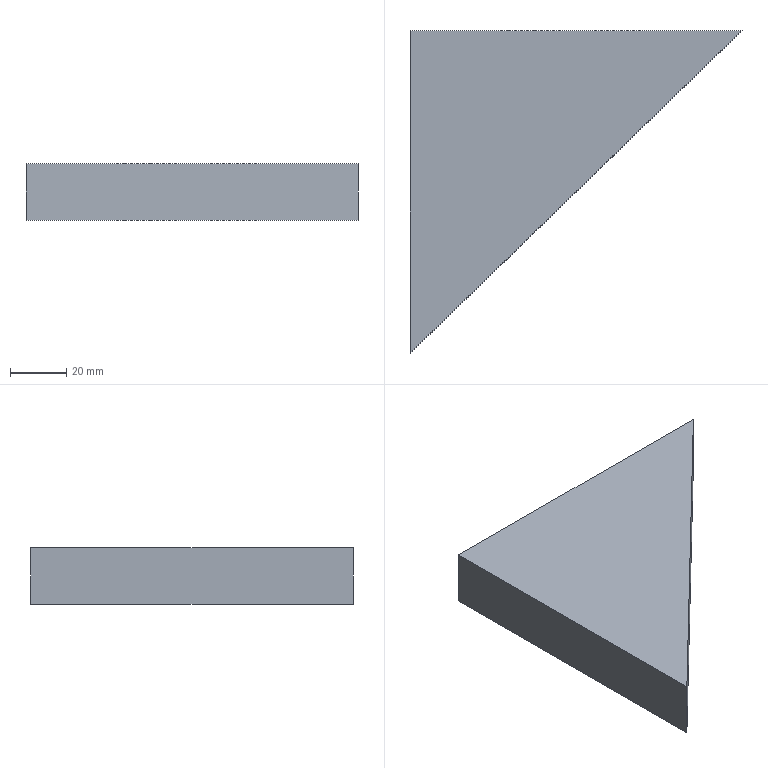Part | STEP file | 1 solid | 5 faces | box 117.801 x 114.536 x 20 mm | volume 134925 mm3 | plane 5
STEP:
#1=CARTESIAN_POINT('',(0.,0.,0.));
#2=DIRECTION('',(0.,0.,1.));
#3=DIRECTION('',(1.,0.,0.));
#4=AXIS2_PLACEMENT_3D('',#1,#2,#3);
#5=CARTESIAN_POINT('',(-480.,430.,-10.));
#6=VERTEX_POINT('',#5);
#7=CARTESIAN_POINT('',(-480.,315.464,-10.));
#8=VERTEX_POINT('',#7);
#9=CARTESIAN_POINT('',(-480.,430.,-10.));
#10=DIRECTION('',(0.,-1.,0.));
#11=VECTOR('',#10,1.);
#12=LINE('',#9,#11);
#13=CARTESIAN_POINT('',(-480.,430.,10.));
#14=DIRECTION('',(1.,0.,0.));
#15=DIRECTION('',(0.,0.,-1.));
#16=AXIS2_PLACEMENT_3D('',#13,#14,#15);
#17=PLANE('',#16);
#18=CARTESIAN_POINT('',(20.,0.));
#19=DIRECTION('',(0.,-1.));
#20=VECTOR('',#19,1.);
#21=LINE('',#18,#20);
#22=(GEOMETRIC_REPRESENTATION_CONTEXT(2)PARAMETRIC_REPRESENTATION_CONTEXT()REPRESENTATION_CONTEXT('',''));
#23=DEFINITIONAL_REPRESENTATION('',(#21),#22);
#24=PCURVE('',#17,#23);
#25=CARTESIAN_POINT('',(0.,0.,-10.));
#26=DIRECTION('',(0.,0.,-1.));
#27=DIRECTION('',(-1.,0.,0.));
#28=AXIS2_PLACEMENT_3D('',#25,#26,#27);
#29=PLANE('',#28);
#30=CARTESIAN_POINT('',(480.,430.));
#31=DIRECTION('',(0.,-1.));
#32=VECTOR('',#31,1.);
#33=LINE('',#30,#32);
#34=(GEOMETRIC_REPRESENTATION_CONTEXT(2)PARAMETRIC_REPRESENTATION_CONTEXT()REPRESENTATION_CONTEXT('',''));
#35=DEFINITIONAL_REPRESENTATION('',(#33),#34);
#36=PCURVE('',#29,#35);
#37=SURFACE_CURVE('',#12,(#24,#36),.PCURVE_S1.);
#38=EDGE_CURVE('',#6,#8,#37,.T.);
#39=ORIENTED_EDGE('',*,*,#38,.T.);
#40=CARTESIAN_POINT('',(-480.,315.464,10.));
#41=VERTEX_POINT('',#40);
#42=CARTESIAN_POINT('',(-480.,315.464,10.));
#43=DIRECTION('',(0.,0.,-1.));
#44=VECTOR('',#43,1.);
#45=LINE('',#42,#44);
#46=CARTESIAN_POINT('',(0.,-114.536));
#47=DIRECTION('',(1.,0.));
#48=VECTOR('',#47,1.);
#49=LINE('',#46,#48);
#50=(GEOMETRIC_REPRESENTATION_CONTEXT(2)PARAMETRIC_REPRESENTATION_CONTEXT()REPRESENTATION_CONTEXT('',''));
#51=DEFINITIONAL_REPRESENTATION('',(#49),#50);
#52=PCURVE('',#17,#51);
#53=CARTESIAN_POINT('',(-480.,315.464,10.));
#54=DIRECTION('',(-0.6971,0.717,0.));
#55=DIRECTION('',(-0.717,-0.6971,0.));
#56=AXIS2_PLACEMENT_3D('',#53,#54,#55);
#57=PLANE('',#56);
#58=CARTESIAN_POINT('',(0.,0.));
#59=DIRECTION('',(0.,-1.));
#60=VECTOR('',#59,1.);
#61=LINE('',#58,#60);
#62=(GEOMETRIC_REPRESENTATION_CONTEXT(2)PARAMETRIC_REPRESENTATION_CONTEXT()REPRESENTATION_CONTEXT('',''));
#63=DEFINITIONAL_REPRESENTATION('',(#61),#62);
#64=PCURVE('',#57,#63);
#65=SURFACE_CURVE('',#45,(#52,#64),.PCURVE_S1.);
#66=EDGE_CURVE('',#41,#8,#65,.T.);
#67=ORIENTED_EDGE('',*,*,#66,.F.);
#68=CARTESIAN_POINT('',(-480.,430.,10.));
#69=VERTEX_POINT('',#68);
#70=CARTESIAN_POINT('',(-480.,430.,10.));
#71=DIRECTION('',(0.,-1.,0.));
#72=VECTOR('',#71,1.);
#73=LINE('',#70,#72);
#74=CARTESIAN_POINT('',(0.,0.));
#75=DIRECTION('',(0.,-1.));
#76=VECTOR('',#75,1.);
#77=LINE('',#74,#76);
#78=(GEOMETRIC_REPRESENTATION_CONTEXT(2)PARAMETRIC_REPRESENTATION_CONTEXT()REPRESENTATION_CONTEXT('',''));
#79=DEFINITIONAL_REPRESENTATION('',(#77),#78);
#80=PCURVE('',#17,#79);
#81=CARTESIAN_POINT('',(0.,0.,10.));
#82=DIRECTION('',(0.,0.,-1.));
#83=DIRECTION('',(-1.,0.,0.));
#84=AXIS2_PLACEMENT_3D('',#81,#82,#83);
#85=PLANE('',#84);
#86=CARTESIAN_POINT('',(480.,430.));
#87=DIRECTION('',(0.,-1.));
#88=VECTOR('',#87,1.);
#89=LINE('',#86,#88);
#90=(GEOMETRIC_REPRESENTATION_CONTEXT(2)PARAMETRIC_REPRESENTATION_CONTEXT()REPRESENTATION_CONTEXT('',''));
#91=DEFINITIONAL_REPRESENTATION('',(#89),#90);
#92=PCURVE('',#85,#91);
#93=SURFACE_CURVE('',#73,(#80,#92),.PCURVE_S1.);
#94=EDGE_CURVE('',#69,#41,#93,.T.);
#95=ORIENTED_EDGE('',*,*,#94,.F.);
#96=CARTESIAN_POINT('',(-480.,430.,10.));
#97=DIRECTION('',(0.,0.,-1.));
#98=VECTOR('',#97,1.);
#99=LINE('',#96,#98);
#100=CARTESIAN_POINT('',(0.,0.));
#101=DIRECTION('',(1.,0.));
#102=VECTOR('',#101,1.);
#103=LINE('',#100,#102);
#104=(GEOMETRIC_REPRESENTATION_CONTEXT(2)PARAMETRIC_REPRESENTATION_CONTEXT()REPRESENTATION_CONTEXT('',''));
#105=DEFINITIONAL_REPRESENTATION('',(#103),#104);
#106=PCURVE('',#17,#105);
#107=CARTESIAN_POINT('',(-362.199,430.,10.));
#108=DIRECTION('',(0.,-1.,0.));
#109=DIRECTION('',(0.,0.,-1.));
#110=AXIS2_PLACEMENT_3D('',#107,#108,#109);
#111=PLANE('',#110);
#112=CARTESIAN_POINT('',(0.,-117.801));
#113=DIRECTION('',(1.,0.));
#114=VECTOR('',#113,1.);
#115=LINE('',#112,#114);
#116=(GEOMETRIC_REPRESENTATION_CONTEXT(2)PARAMETRIC_REPRESENTATION_CONTEXT()REPRESENTATION_CONTEXT('',''));
#117=DEFINITIONAL_REPRESENTATION('',(#115),#116);
#118=PCURVE('',#111,#117);
#119=SURFACE_CURVE('',#99,(#106,#118),.PCURVE_S1.);
#120=EDGE_CURVE('',#69,#6,#119,.T.);
#121=ORIENTED_EDGE('',*,*,#120,.T.);
#122=EDGE_LOOP('',(#39,#67,#95,#121));
#123=FACE_BOUND('',#122,.T.);
#124=ADVANCED_FACE('',(#123),#17,.F.);
#125=CARTESIAN_POINT('',(-362.199,430.,-10.));
#126=VERTEX_POINT('',#125);
#127=CARTESIAN_POINT('',(-480.,315.464,-10.));
#128=DIRECTION('',(0.717,0.6971,0.));
#129=VECTOR('',#128,1.);
#130=LINE('',#127,#129);
#131=CARTESIAN_POINT('',(0.,-20.));
#132=DIRECTION('',(-1.,0.));
#133=VECTOR('',#132,1.);
#134=LINE('',#131,#133);
#135=(GEOMETRIC_REPRESENTATION_CONTEXT(2)PARAMETRIC_REPRESENTATION_CONTEXT()REPRESENTATION_CONTEXT('',''));
#136=DEFINITIONAL_REPRESENTATION('',(#134),#135);
#137=PCURVE('',#57,#136);
#138=CARTESIAN_POINT('',(480.,315.464));
#139=DIRECTION('',(-0.717,0.6971));
#140=VECTOR('',#139,1.);
#141=LINE('',#138,#140);
#142=(GEOMETRIC_REPRESENTATION_CONTEXT(2)PARAMETRIC_REPRESENTATION_CONTEXT()REPRESENTATION_CONTEXT('',''));
#143=DEFINITIONAL_REPRESENTATION('',(#141),#142);
#144=PCURVE('',#29,#143);
#145=SURFACE_CURVE('',#130,(#137,#144),.PCURVE_S1.);
#146=EDGE_CURVE('',#8,#126,#145,.T.);
#147=ORIENTED_EDGE('',*,*,#146,.T.);
#148=CARTESIAN_POINT('',(-362.199,430.,10.));
#149=VERTEX_POINT('',#148);
#150=CARTESIAN_POINT('',(-362.199,430.,10.));
#151=DIRECTION('',(0.,0.,-1.));
#152=VECTOR('',#151,1.);
#153=LINE('',#150,#152);
#154=CARTESIAN_POINT('',(-164.304,0.));
#155=DIRECTION('',(0.,-1.));
#156=VECTOR('',#155,1.);
#157=LINE('',#154,#156);
#158=(GEOMETRIC_REPRESENTATION_CONTEXT(2)PARAMETRIC_REPRESENTATION_CONTEXT()REPRESENTATION_CONTEXT('',''));
#159=DEFINITIONAL_REPRESENTATION('',(#157),#158);
#160=PCURVE('',#57,#159);
#161=CARTESIAN_POINT('',(0.,0.));
#162=DIRECTION('',(1.,0.));
#163=VECTOR('',#162,1.);
#164=LINE('',#161,#163);
#165=(GEOMETRIC_REPRESENTATION_CONTEXT(2)PARAMETRIC_REPRESENTATION_CONTEXT()REPRESENTATION_CONTEXT('',''));
#166=DEFINITIONAL_REPRESENTATION('',(#164),#165);
#167=PCURVE('',#111,#166);
#168=SURFACE_CURVE('',#153,(#160,#167),.PCURVE_S1.);
#169=EDGE_CURVE('',#149,#126,#168,.T.);
#170=ORIENTED_EDGE('',*,*,#169,.F.);
#171=CARTESIAN_POINT('',(-480.,315.464,10.));
#172=DIRECTION('',(0.717,0.6971,0.));
#173=VECTOR('',#172,1.);
#174=LINE('',#171,#173);
#175=CARTESIAN_POINT('',(0.,0.));
#176=DIRECTION('',(-1.,0.));
#177=VECTOR('',#176,1.);
#178=LINE('',#175,#177);
#179=(GEOMETRIC_REPRESENTATION_CONTEXT(2)PARAMETRIC_REPRESENTATION_CONTEXT()REPRESENTATION_CONTEXT('',''));
#180=DEFINITIONAL_REPRESENTATION('',(#178),#179);
#181=PCURVE('',#57,#180);
#182=CARTESIAN_POINT('',(480.,315.464));
#183=DIRECTION('',(-0.717,0.6971));
#184=VECTOR('',#183,1.);
#185=LINE('',#182,#184);
#186=(GEOMETRIC_REPRESENTATION_CONTEXT(2)PARAMETRIC_REPRESENTATION_CONTEXT()REPRESENTATION_CONTEXT('',''));
#187=DEFINITIONAL_REPRESENTATION('',(#185),#186);
#188=PCURVE('',#85,#187);
#189=SURFACE_CURVE('',#174,(#181,#188),.PCURVE_S1.);
#190=EDGE_CURVE('',#41,#149,#189,.T.);
#191=ORIENTED_EDGE('',*,*,#190,.F.);
#192=ORIENTED_EDGE('',*,*,#66,.T.);
#193=EDGE_LOOP('',(#147,#170,#191,#192));
#194=FACE_BOUND('',#193,.T.);
#195=ADVANCED_FACE('',(#194),#57,.F.);
#196=CARTESIAN_POINT('',(-362.199,430.,-10.));
#197=DIRECTION('',(-1.,0.,0.));
#198=VECTOR('',#197,1.);
#199=LINE('',#196,#198);
#200=CARTESIAN_POINT('',(20.,0.));
#201=DIRECTION('',(0.,-1.));
#202=VECTOR('',#201,1.);
#203=LINE('',#200,#202);
#204=(GEOMETRIC_REPRESENTATION_CONTEXT(2)PARAMETRIC_REPRESENTATION_CONTEXT()REPRESENTATION_CONTEXT('',''));
#205=DEFINITIONAL_REPRESENTATION('',(#203),#204);
#206=PCURVE('',#111,#205);
#207=CARTESIAN_POINT('',(362.199,430.));
#208=DIRECTION('',(1.,0.));
#209=VECTOR('',#208,1.);
#210=LINE('',#207,#209);
#211=(GEOMETRIC_REPRESENTATION_CONTEXT(2)PARAMETRIC_REPRESENTATION_CONTEXT()REPRESENTATION_CONTEXT('',''));
#212=DEFINITIONAL_REPRESENTATION('',(#210),#211);
#213=PCURVE('',#29,#212);
#214=SURFACE_CURVE('',#199,(#206,#213),.PCURVE_S1.);
#215=EDGE_CURVE('',#126,#6,#214,.T.);
#216=ORIENTED_EDGE('',*,*,#215,.T.);
#217=ORIENTED_EDGE('',*,*,#120,.F.);
#218=CARTESIAN_POINT('',(-362.199,430.,10.));
#219=DIRECTION('',(-1.,0.,0.));
#220=VECTOR('',#219,1.);
#221=LINE('',#218,#220);
#222=CARTESIAN_POINT('',(0.,0.));
#223=DIRECTION('',(0.,-1.));
#224=VECTOR('',#223,1.);
#225=LINE('',#222,#224);
#226=(GEOMETRIC_REPRESENTATION_CONTEXT(2)PARAMETRIC_REPRESENTATION_CONTEXT()REPRESENTATION_CONTEXT('',''));
#227=DEFINITIONAL_REPRESENTATION('',(#225),#226);
#228=PCURVE('',#111,#227);
#229=CARTESIAN_POINT('',(362.199,430.));
#230=DIRECTION('',(1.,0.));
#231=VECTOR('',#230,1.);
#232=LINE('',#229,#231);
#233=(GEOMETRIC_REPRESENTATION_CONTEXT(2)PARAMETRIC_REPRESENTATION_CONTEXT()REPRESENTATION_CONTEXT('',''));
#234=DEFINITIONAL_REPRESENTATION('',(#232),#233);
#235=PCURVE('',#85,#234);
#236=SURFACE_CURVE('',#221,(#228,#235),.PCURVE_S1.);
#237=EDGE_CURVE('',#149,#69,#236,.T.);
#238=ORIENTED_EDGE('',*,*,#237,.F.);
#239=ORIENTED_EDGE('',*,*,#169,.T.);
#240=EDGE_LOOP('',(#216,#217,#238,#239));
#241=FACE_BOUND('',#240,.T.);
#242=ADVANCED_FACE('',(#241),#111,.F.);
#243=ORIENTED_EDGE('',*,*,#94,.T.);
#244=ORIENTED_EDGE('',*,*,#190,.T.);
#245=ORIENTED_EDGE('',*,*,#237,.T.);
#246=EDGE_LOOP('',(#243,#244,#245));
#247=FACE_BOUND('',#246,.T.);
#248=ADVANCED_FACE('',(#247),#85,.F.);
#249=ORIENTED_EDGE('',*,*,#38,.F.);
#250=ORIENTED_EDGE('',*,*,#215,.F.);
#251=ORIENTED_EDGE('',*,*,#146,.F.);
#252=EDGE_LOOP('',(#249,#250,#251));
#253=FACE_BOUND('',#252,.T.);
#254=ADVANCED_FACE('',(#253),#29,.T.);
#255=CLOSED_SHELL('',(#124,#195,#242,#248,#254));
#256=MANIFOLD_SOLID_BREP('',#255);
#257=(LENGTH_UNIT()NAMED_UNIT(*)SI_UNIT(.MILLI.,.METRE.));
#258=UNCERTAINTY_MEASURE_WITH_UNIT(LENGTH_MEASURE(0.0000001),#257,'','');
#259=(NAMED_UNIT(*)PLANE_ANGLE_UNIT()SI_UNIT($,.RADIAN.));
#260=(NAMED_UNIT(*)SI_UNIT($,.STERADIAN.)SOLID_ANGLE_UNIT());
#261=(GEOMETRIC_REPRESENTATION_CONTEXT(3)GLOBAL_UNCERTAINTY_ASSIGNED_CONTEXT((#258))GLOBAL_UNIT_ASSIGNED_CONTEXT((#257,#259,#260))REPRESENTATION_CONTEXT('',''));
#262=ADVANCED_BREP_SHAPE_REPRESENTATION('',(#4,#256),#261);